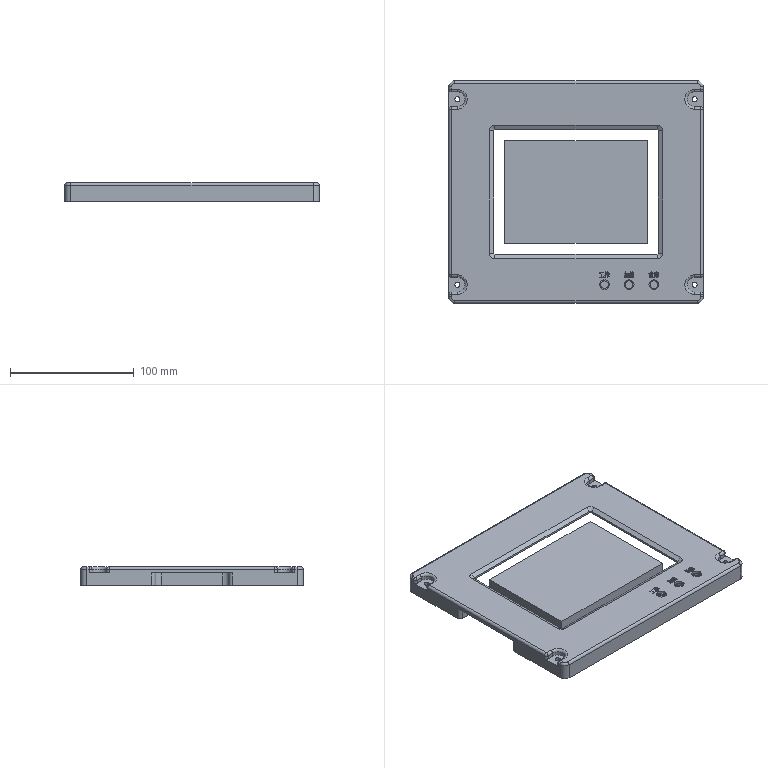NC program | Mastercam | posted with a generic post | part box 206 x 180 x 15 mm
Lines 1 to 736 of 42274:
%
:0001()
(MATERIAL - ALUMINUM MM - 2024)
(T24|100 FEM |H24)
(T9|10 FEM |H9|XY STOCK TO LEAVE - .15|Z STOCK TO LEAVE - .05)
(T10|10 FEM |H10)
(T1|4 BNOS |H1|XY STOCK TO LEAVE - .1|Z STOCK TO LEAVE - 0.)
(T14|2 BM/BNOS |H14)
(T4|4 FEM |H4|XY STOCK TO LEAVE - -.01|Z STOCK TO LEAVE - 0.)
(T8|8 FEM |H8|XY STOCK TO LEAVE - 0.|Z STOCK TO LEAVE - .1)
(T5|4 CHM |H5)
(T2|2 FEM |H2|XY STOCK TO LEAVE - .1|Z STOCK TO LEAVE - 0.)
N100 G21
N102 G0 G17 G40 G80 G90 G94 G98
N104 G0 G28 G91 Z0.
N106 G0 G28 X0. Y0.
(100 FEM |TOOL - 24|DIA. OFF. - 24|LEN. - 24|TOOL DIA. - 100.)
N108 T24 M6
N110 G0 G54 G90 X-215.5 Y64.998 C0. B0. S4000 M3
N112 G43 H24 Z51.
N114 Z3.
N116 G1 Z.55 F600.
N118 X155.5 F1000.
N120 G2 X187.999 Y32.499 J-32.499
N122 X155.5 Y0. I-32.499
N124 G1 X-155.5
N126 G3 X-187.999 Y-32.499 J-32.499
N128 X-155.5 Y-64.998 I32.499
N130 G1 X215.5
N132 G0 Z50.55
N134 X-215.5 Y64.998
N136 Z2.55
N138 G1 Z.1 F600.
N140 X155.5 F1000.
N142 G2 X187.999 Y32.499 J-32.499
N144 X155.5 Y0. I-32.499
N146 G1 X-155.5
N148 G3 X-187.999 Y-32.499 J-32.499
N150 X-155.5 Y-64.998 I32.499
N152 G1 X215.5
N154 G0 Z50.1
N156 X-215.5 Y64.998
N158 Z2.1
N160 G1 Z0. F600.
N162 X155.5 F1000.
N164 G2 X187.999 Y32.499 J-32.499
N166 X155.5 Y0. I-32.499
N168 G1 X-155.5
N170 G3 X-187.999 Y-32.499 J-32.499
N172 X-155.5 Y-64.998 I32.499
N174 G1 X215.5
N176 G0 Z50.
N178 M5
N180 G0 G28 G91 Z0.
N182 G28
N184 M01
N186 G0 G17 G40 G80 G90 G94 G98
N188 G0 G28 G91 Z0.
(10 FEM |TOOL - 9|DIA. OFF. - 9|LEN. - 9|TOOL DIA. - 10.)
N190 T9 M6
N192 G0 G54 G90 X-99. Y97.15 C0. B0. S7000 M3
N194 G43 H9 Z50.
N196 Z1.
N198 G1 Z0. F600.
N200 Y96.15 F3000.
N202 G3 X-98. Y95.15 I1.
N204 G1 X98. Z-.246
N206 G2 X108.15 Y85. Z-.266 J-10.15
N208 G1 Y-85. Z-.48
N210 G2 X98. Y-95.15 Z-.5 I-10.15
N212 G1 X-98. Z-.746
N214 G2 X-108.15 Y-85. Z-.766 J10.15
N216 G1 Y85. Z-.98
N218 G2 X-98. Y95.15 Z-1. I10.15
N220 G1 X98. Z-1.246
N222 G2 X108.15 Y85. Z-1.266 J-10.15
N224 G1 Y-85. Z-1.48
N226 G2 X98. Y-95.15 Z-1.5 I-10.15
N228 G1 X-98. Z-1.746
N230 G2 X-108.15 Y-85. Z-1.766 J10.15
N232 G1 Y85. Z-1.98
N234 G2 X-98. Y95.15 Z-2. I10.15
N236 G1 X98. Z-2.246
N238 G2 X108.15 Y85. Z-2.266 J-10.15
N240 G1 Y-85. Z-2.48
N242 G2 X98. Y-95.15 Z-2.5 I-10.15
N244 G1 X-98. Z-2.746
N246 G2 X-108.15 Y-85. Z-2.766 J10.15
N248 G1 Y85. Z-2.98
N250 G2 X-98. Y95.15 Z-3. I10.15
N252 G1 X98. Z-3.246
N254 G2 X108.15 Y85. Z-3.266 J-10.15
N256 G1 Y-85. Z-3.48
N258 G2 X98. Y-95.15 Z-3.5 I-10.15
N260 G1 X-98. Z-3.746
N262 G2 X-108.15 Y-85. Z-3.766 J10.15
N264 G1 Y85. Z-3.98
N266 G2 X-98. Y95.15 Z-4. I10.15
N268 G1 X98. Z-4.246
N270 G2 X108.15 Y85. Z-4.266 J-10.15
N272 G1 Y-85. Z-4.48
N274 G2 X98. Y-95.15 Z-4.5 I-10.15
N276 G1 X-98. Z-4.746
N278 G2 X-108.15 Y-85. Z-4.766 J10.15
N280 G1 Y85. Z-4.98
N282 G2 X-98. Y95.15 Z-5. I10.15
N284 G1 X98. Z-5.246
N286 G2 X108.15 Y85. Z-5.266 J-10.15
N288 G1 Y-85. Z-5.48
N290 G2 X98. Y-95.15 Z-5.5 I-10.15
N292 G1 X-98. Z-5.746
N294 G2 X-108.15 Y-85. Z-5.766 J10.15
N296 G1 Y85. Z-5.98
N298 G2 X-98. Y95.15 Z-6. I10.15
N300 G1 X98. Z-6.246
N302 G2 X108.15 Y85. Z-6.266 J-10.15
N304 G1 Y-85. Z-6.48
N306 G2 X98. Y-95.15 Z-6.5 I-10.15
N308 G1 X-98. Z-6.746
N310 G2 X-108.15 Y-85. Z-6.766 J10.15
N312 G1 Y85. Z-6.98
N314 G2 X-98. Y95.15 Z-7. I10.15
N316 G1 X98. Z-7.246
N318 G2 X108.15 Y85. Z-7.266 J-10.15
N320 G1 Y-85. Z-7.48
N322 G2 X98. Y-95.15 Z-7.5 I-10.15
N324 G1 X-98. Z-7.746
N326 G2 X-108.15 Y-85. Z-7.766 J10.15
N328 G1 Y85. Z-7.98
N330 G2 X-98. Y95.15 Z-8. I10.15
N332 G1 X98. Z-8.246
N334 G2 X108.15 Y85. Z-8.266 J-10.15
N336 G1 Y-85. Z-8.48
N338 G2 X98. Y-95.15 Z-8.5 I-10.15
N340 G1 X-98. Z-8.746
N342 G2 X-108.15 Y-85. Z-8.766 J10.15
N344 G1 Y85. Z-8.98
N346 G2 X-98. Y95.15 Z-9. I10.15
N348 G1 X98. Z-9.246
N350 G2 X108.15 Y85. Z-9.266 J-10.15
N352 G1 Y-85. Z-9.48
N354 G2 X98. Y-95.15 Z-9.5 I-10.15
N356 G1 X-98. Z-9.746
N358 G2 X-108.15 Y-85. Z-9.766 J10.15
N360 G1 Y85. Z-9.98
N362 G2 X-98. Y95.15 Z-10. I10.15
N364 G1 X98. Z-10.246
N366 G2 X108.15 Y85. Z-10.266 J-10.15
N368 G1 Y-85. Z-10.48
N370 G2 X98. Y-95.15 Z-10.5 I-10.15
N372 G1 X-98. Z-10.746
N374 G2 X-108.15 Y-85. Z-10.766 J10.15
N376 G1 Y85. Z-10.98
N378 G2 X-98. Y95.15 Z-11. I10.15
N380 G1 X98. Z-11.246
N382 G2 X108.15 Y85. Z-11.266 J-10.15
N384 G1 Y-85. Z-11.48
N386 G2 X98. Y-95.15 Z-11.5 I-10.15
N388 G1 X-98. Z-11.746
N390 G2 X-108.15 Y-85. Z-11.766 J10.15
N392 G1 Y85. Z-11.98
N394 G2 X-98. Y95.15 Z-12. I10.15
N396 G1 X98. Z-12.246
N398 G2 X108.15 Y85. Z-12.266 J-10.15
N400 G1 Y-85. Z-12.48
N402 G2 X98. Y-95.15 Z-12.5 I-10.15
N404 G1 X-98. Z-12.746
N406 G2 X-108.15 Y-85. Z-12.766 J10.15
N408 G1 Y85. Z-12.98
N410 G2 X-98. Y95.15 Z-13. I10.15
N412 G1 X98. Z-13.246
N414 G2 X108.15 Y85. Z-13.266 J-10.15
N416 G1 Y-85. Z-13.48
N418 G2 X98. Y-95.15 Z-13.5 I-10.15
N420 G1 X-98. Z-13.746
N422 G2 X-108.15 Y-85. Z-13.766 J10.15
N424 G1 Y85. Z-13.98
N426 G2 X-98. Y95.15 Z-14. I10.15
N428 G1 X98. Z-14.246
N430 G2 X108.15 Y85. Z-14.266 J-10.15
N432 G1 Y-85. Z-14.48
N434 G2 X98. Y-95.15 Z-14.5 I-10.15
N436 G1 X-98. Z-14.746
N438 G2 X-108.15 Y-85. Z-14.766 J10.15
N440 G1 Y61.155 Z-14.95
N442 Y85.
N444 G2 X-98. Y95.15 I10.15
N446 G1 X98.
N448 G2 X108.15 Y85. J-10.15
N450 G1 Y-85.
N452 G2 X98. Y-95.15 I-10.15
N454 G1 X-98.
N456 G2 X-108.15 Y-85. J10.15
N458 G1 Y61.155
N460 G3 X-109.15 Y62.155 I-1.
N462 G1 X-110.15
N464 G0 Z50.
N466 X-110.1 Y66.
N468 Z1.
N470 G1 Z-.485 F600.
N472 X-109.1 F3000.
N474 G3 X-108.1 Y67. J1.
N476 G2 X-101. Y74.1 I7.1
N478 G1 X-96.
N480 G3 X-95.1 Y75. J.9
N482 X-96. Y75.9 I-.9
N484 G1 X-101.
N486 G2 X-108.1 Y83. J7.1
N488 G3 X-109.1 Y84. I-1.
N490 G1 X-110.1
N492 Z-.97 F600.
N494 X-109.1 F3000.
N496 G2 X-108.1 Y83. J-1.
N498 G3 X-101. Y75.9 I7.1
N500 G1 X-96.
N502 G2 X-95.1 Y75. J-.9
N504 X-96. Y74.1 I-.9
N506 G1 X-101.
N508 G3 X-108.1 Y67. J-7.1
N510 G2 X-109.1 Y66. I-1.
N512 G1 X-110.1
N514 Z-1.455 F600.
N516 X-109.1 F3000.
N518 G3 X-108.1 Y67. J1.
N520 G2 X-101. Y74.1 I7.1
N522 G1 X-96.
N524 G3 X-95.1 Y75. J.9
N526 X-96. Y75.9 I-.9
N528 G1 X-101.
N530 G2 X-108.1 Y83. J7.1
N532 G3 X-109.1 Y84. I-1.
N534 G1 X-110.1
N536 Z-1.94 F600.
N538 X-109.1 F3000.
N540 G2 X-108.1 Y83. J-1.
N542 G3 X-101. Y75.9 I7.1
N544 G1 X-96.
N546 G2 X-95.1 Y75. J-.9
N548 X-96. Y74.1 I-.9
N550 G1 X-101.
N552 G3 X-108.1 Y67. J-7.1
N554 G2 X-109.1 Y66. I-1.
N556 G1 X-110.1
N558 Z-2.425 F600.
N560 X-109.1 F3000.
N562 G3 X-108.1 Y67. J1.
N564 G2 X-101. Y74.1 I7.1
N566 G1 X-96.
N568 G3 X-95.1 Y75. J.9
N570 X-96. Y75.9 I-.9
N572 G1 X-101.
N574 G2 X-108.1 Y83. J7.1
N576 G3 X-109.1 Y84. I-1.
N578 G1 X-110.1
N580 Z-2.91 F600.
N582 X-109.1 F3000.
N584 G2 X-108.1 Y83. J-1.
N586 G3 X-101. Y75.9 I7.1
N588 G1 X-96.
N590 G2 X-95.1 Y75. J-.9
N592 X-96. Y74.1 I-.9
N594 G1 X-101.
N596 G3 X-108.1 Y67. J-7.1
N598 G2 X-109.1 Y66. I-1.
N600 G1 X-110.1
N602 Z-3.395 F600.
N604 X-109.1 F3000.
N606 G3 X-108.1 Y67. J1.
N608 G2 X-101. Y74.1 I7.1
N610 G1 X-96.
N612 G3 X-95.1 Y75. J.9
N614 X-96. Y75.9 I-.9
N616 G1 X-101.
N618 G2 X-108.1 Y83. J7.1
N620 G3 X-109.1 Y84. I-1.
N622 G1 X-110.1
N624 Z-3.88 F600.
N626 X-109.1 F3000.
N628 G2 X-108.1 Y83. J-1.
N630 G3 X-101. Y75.9 I7.1
N632 G1 X-96.
N634 G2 X-95.1 Y75. J-.9
N636 X-96. Y74.1 I-.9
N638 G1 X-101.
N640 G3 X-108.1 Y67. J-7.1
N642 G2 X-109.1 Y66. I-1.
N644 G1 X-110.1
N646 Z-4.365 F600.
N648 X-109.1 F3000.
N650 G3 X-108.1 Y67. J1.
N652 G2 X-101. Y74.1 I7.1
N654 G1 X-96.
N656 G3 X-95.1 Y75. J.9
N658 X-96. Y75.9 I-.9
N660 G1 X-101.
N662 G2 X-108.1 Y83. J7.1
N664 G3 X-109.1 Y84. I-1.
N666 G1 X-110.1
N668 Z-4.85 F600.
N670 X-109.1 F3000.
N672 G2 X-108.1 Y83. J-1.
N674 G3 X-101. Y75.9 I7.1
N676 G1 X-96.
N678 G2 X-95.1 Y75. J-.9
N680 X-96. Y74.1 I-.9
N682 G1 X-101.
N684 G3 X-108.1 Y67. J-7.1
N686 G2 X-109.1 Y66. I-1.
N688 G1 X-110.1
N690 G0 Z50.
N692 Y-84.
N694 Z1.
N696 G1 Z-.485 F600.
N698 X-109.1 F3000.
N700 G3 X-108.1 Y-83. J1.
N702 G2 X-101. Y-75.9 I7.1
N704 G1 X-96.
N706 G3 X-95.1 Y-75. J.9
N708 X-96. Y-74.1 I-.9
N710 G1 X-101.
N712 G2 X-108.1 Y-67. J7.1
N714 G3 X-109.1 Y-66. I-1.
N716 G1 X-110.1
N718 Z-.97 F600.
N720 X-109.1 F3000.
N722 G2 X-108.1 Y-67. J-1.
N724 G3 X-101. Y-74.1 I7.1
N726 G1 X-96.
N728 G2 X-95.1 Y-75. J-.9
N730 X-96. Y-75.9 I-.9
N732 G1 X-101.
N734 G3 X-108.1 Y-83. J-7.1
N736 G2 X-109.1 Y-84. I-1.
N738 G1 X-110.1
N740 Z-1.455 F600.
N742 X-109.1 F3000.
N744 G3 X-108.1 Y-83. J1.
N746 G2 X-101. Y-75.9 I7.1
N748 G1 X-96.
N750 G3 X-95.1 Y-75. J.9
N752 X-96. Y-74.1 I-.9
N754 G1 X-101.
N756 G2 X-108.1 Y-67. J7.1
N758 G3 X-109.1 Y-66. I-1.
N760 G1 X-110.1
N762 Z-1.94 F600.
N764 X-109.1 F3000.
N766 G2 X-108.1 Y-67. J-1.
N768 G3 X-101. Y-74.1 I7.1
N770 G1 X-96.
N772 G2 X-95.1 Y-75. J-.9
N774 X-96. Y-75.9 I-.9
N776 G1 X-101.
N778 G3 X-108.1 Y-83. J-7.1
N780 G2 X-109.1 Y-84. I-1.
N782 G1 X-110.1
N784 Z-2.425 F600.
N786 X-109.1 F3000.
N788 G3 X-108.1 Y-83. J1.
N790 G2 X-101. Y-75.9 I7.1
N792 G1 X-96.
N794 G3 X-95.1 Y-75. J.9
N796 X-96. Y-74.1 I-.9
N798 G1 X-101.
N800 G2 X-108.1 Y-67. J7.1
N802 G3 X-109.1 Y-66. I-1.
N804 G1 X-110.1
N806 Z-2.91 F600.
N808 X-109.1 F3000.
N810 G2 X-108.1 Y-67. J-1.
N812 G3 X-101. Y-74.1 I7.1
N814 G1 X-96.
N816 G2 X-95.1 Y-75. J-.9
N818 X-96. Y-75.9 I-.9
N820 G1 X-101.
N822 G3 X-108.1 Y-83. J-7.1
N824 G2 X-109.1 Y-84. I-1.
N826 G1 X-110.1
N828 Z-3.395 F600.
N830 X-109.1 F3000.
N832 G3 X-108.1 Y-83. J1.
N834 G2 X-101. Y-75.9 I7.1
N836 G1 X-96.
N838 G3 X-95.1 Y-75. J.9
N840 X-96. Y-74.1 I-.9
N842 G1 X-101.
N844 G2 X-108.1 Y-67. J7.1
N846 G3 X-109.1 Y-66. I-1.
N848 G1 X-110.1
N850 Z-3.88 F600.
N852 X-109.1 F3000.
N854 G2 X-108.1 Y-67. J-1.
N856 G3 X-101. Y-74.1 I7.1
N858 G1 X-96.
N860 G2 X-95.1 Y-75. J-.9
N862 X-96. Y-75.9 I-.9
N864 G1 X-101.
N866 G3 X-108.1 Y-83. J-7.1
N868 G2 X-109.1 Y-84. I-1.
N870 G1 X-110.1
N872 Z-4.365 F600.
N874 X-109.1 F3000.
N876 G3 X-108.1 Y-83. J1.
N878 G2 X-101. Y-75.9 I7.1
N880 G1 X-96.
N882 G3 X-95.1 Y-75. J.9
N884 X-96. Y-74.1 I-.9
N886 G1 X-101.
N888 G2 X-108.1 Y-67. J7.1
N890 G3 X-109.1 Y-66. I-1.
N892 G1 X-110.1
N894 Z-4.85 F600.
N896 X-109.1 F3000.
N898 G2 X-108.1 Y-67. J-1.
N900 G3 X-101. Y-74.1 I7.1
N902 G1 X-96.
N904 G2 X-95.1 Y-75. J-.9
N906 X-96. Y-75.9 I-.9
N908 G1 X-101.
N910 G3 X-108.1 Y-83. J-7.1
N912 G2 X-109.1 Y-84. I-1.
N914 G1 X-110.1
N916 G0 Z50.
N918 X110.1 Y-66.
N920 Z1.
N922 G1 Z-.485 F600.
N924 X109.1 F3000.
N926 G3 X108.1 Y-67. J-1.
N928 G2 X101. Y-74.1 I-7.1
N930 G1 X96.
N932 G3 X95.1 Y-75. J-.9
N934 X96. Y-75.9 I.9
N936 G1 X101.
N938 G2 X108.1 Y-83. J-7.1
N940 G3 X109.1 Y-84. I1.
N942 G1 X110.1
N944 Z-.97 F600.
N946 X109.1 F3000.
N948 G2 X108.1 Y-83. J1.
N950 G3 X101. Y-75.9 I-7.1
N952 G1 X96.
N954 G2 X95.1 Y-75. J.9
N956 X96. Y-74.1 I.9
N958 G1 X101.
N960 G3 X108.1 Y-67. J7.1
N962 G2 X109.1 Y-66. I1.
N964 G1 X110.1
N966 Z-1.455 F600.
N968 X109.1 F3000.
N970 G3 X108.1 Y-67. J-1.
N972 G2 X101. Y-74.1 I-7.1
N974 G1 X96.
N976 G3 X95.1 Y-75. J-.9
N978 X96. Y-75.9 I.9
N980 G1 X101.
N982 G2 X108.1 Y-83. J-7.1
N984 G3 X109.1 Y-84. I1.
N986 G1 X110.1
N988 Z-1.94 F600.
N990 X109.1 F3000.
N992 G2 X108.1 Y-83. J1.
N994 G3 X101. Y-75.9 I-7.1
N996 G1 X96.
N998 G2 X95.1 Y-75. J.9
N1000 X96. Y-74.1 I.9
N1002 G1 X101.
N1004 G3 X108.1 Y-67. J7.1
N1006 G2 X109.1 Y-66. I1.
N1008 G1 X110.1
N1010 Z-2.425 F600.
N1012 X109.1 F3000.
N1014 G3 X108.1 Y-67. J-1.
N1016 G2 X101. Y-74.1 I-7.1
N1018 G1 X96.
N1020 G3 X95.1 Y-75. J-.9
N1022 X96. Y-75.9 I.9
N1024 G1 X101.
N1026 G2 X108.1 Y-83. J-7.1
N1028 G3 X109.1 Y-84. I1.
N1030 G1 X110.1
N1032 Z-2.91 F600.
N1034 X109.1 F3000.
N1036 G2 X108.1 Y-83. J1.
N1038 G3 X101. Y-75.9 I-7.1
N1040 G1 X96.
N1042 G2 X95.1 Y-75. J.9
N1044 X96. Y-74.1 I.9
N1046 G1 X101.
N1048 G3 X108.1 Y-67. J7.1
N1050 G2 X109.1 Y-66. I1.
N1052 G1 X110.1
N1054 Z-3.395 F600.
N1056 X109.1 F3000.
N1058 G3 X108.1 Y-67. J-1.
N1060 G2 X101. Y-74.1 I-7.1
N1062 G1 X96.
N1064 G3 X95.1 Y-75. J-.9
N1066 X96. Y-75.9 I.9
N1068 G1 X101.
N1070 G2 X108.1 Y-83. J-7.1
N1072 G3 X109.1 Y-84. I1.
N1074 G1 X110.1
N1076 Z-3.88 F600.
N1078 X109.1 F3000.
N1080 G2 X108.1 Y-83. J1.
N1082 G3 X101. Y-75.9 I-7.1
N1084 G1 X96.
N1086 G2 X95.1 Y-75. J.9
N1088 X96. Y-74.1 I.9
N1090 G1 X101.
N1092 G3 X108.1 Y-67. J7.1
N1094 G2 X109.1 Y-66. I1.
N1096 G1 X110.1
N1098 Z-4.365 F600.
N1100 X109.1 F3000.
N1102 G3 X108.1 Y-67. J-1.
N1104 G2 X101. Y-74.1 I-7.1
N1106 G1 X96.
N1108 G3 X95.1 Y-75. J-.9
N1110 X96. Y-75.9 I.9
N1112 G1 X101.
N1114 G2 X108.1 Y-83. J-7.1
N1116 G3 X109.1 Y-84. I1.
N1118 G1 X110.1
N1120 Z-4.85 F600.
N1122 X109.1 F3000.
N1124 G2 X108.1 Y-83. J1.
N1126 G3 X101. Y-75.9 I-7.1
N1128 G1 X96.
N1130 G2 X95.1 Y-75. J.9
N1132 X96. Y-74.1 I.9
N1134 G1 X101.
N1136 G3 X108.1 Y-67. J7.1
N1138 G2 X109.1 Y-66. I1.
N1140 G1 X110.1
N1142 G0 Z50.
N1144 Y84.
N1146 Z1.
N1148 G1 Z-.485 F600.
N1150 X109.1 F3000.
N1152 G3 X108.1 Y83. J-1.
N1154 G2 X101. Y75.9 I-7.1
N1156 G1 X96.
N1158 G3 X95.1 Y75. J-.9
N1160 X96. Y74.1 I.9
N1162 G1 X101.
N1164 G2 X108.1 Y67. J-7.1
N1166 G3 X109.1 Y66. I1.
N1168 G1 X110.1
N1170 Z-.97 F600.
N1172 X109.1 F3000.
N1174 G2 X108.1 Y67. J1.
N1176 G3 X101. Y74.1 I-7.1
N1178 G1 X96.
N1180 G2 X95.1 Y75. J.9
N1182 X96. Y75.9 I.9
N1184 G1 X101.
N1186 G3 X108.1 Y83. J7.1
N1188 G2 X109.1 Y84. I1.
N1190 G1 X110.1
N1192 Z-1.455 F600.
N1194 X109.1 F3000.
N1196 G3 X108.1 Y83. J-1.
N1198 G2 X101. Y75.9 I-7.1
N1200 G1 X96.
N1202 G3 X95.1 Y75. J-.9
N1204 X96. Y74.1 I.9
N1206 G1 X101.
N1208 G2 X108.1 Y67. J-7.1
N1210 G3 X109.1 Y66. I1.
N1212 G1 X110.1
N1214 Z-1.94 F600.
N1216 X109.1 F3000.
N1218 G2 X108.1 Y67. J1.
N1220 G3 X101. Y74.1 I-7.1
N1222 G1 X96.
N1224 G2 X95.1 Y75. J.9
N1226 X96. Y75.9 I.9
N1228 G1 X101.
N1230 G3 X108.1 Y83. J7.1
N1232 G2 X109.1 Y84. I1.
N1234 G1 X110.1
N1236 Z-2.425 F600.
N1238 X109.1 F3000.
N1240 G3 X108.1 Y83. J-1.
N1242 G2 X101. Y75.9 I-7.1
N1244 G1 X96.
N1246 G3 X95.1 Y75. J-.9
N1248 X96. Y74.1 I.9
N1250 G1 X101.
N1252 G2 X108.1 Y67. J-7.1
N1254 G3 X109.1 Y66. I1.
N1256 G1 X110.1
N1258 Z-2.91 F600.
N1260 X109.1 F3000.
N1262 G2 X108.1 Y67. J1.
N1264 G3 X101. Y74.1 I-7.1
N1266 G1 X96.
N1268 G2 X95.1 Y75. J.9
N1270 X96. Y75.9 I.9
N1272 G1 X101.
N1274 G3 X108.1 Y83. J7.1
N1276 G2 X109.1 Y84. I1.
N1278 G1 X110.1
N1280 Z-3.395 F600.
N1282 X109.1 F3000.
N1284 G3 X108.1 Y83. J-1.
N1286 G2 X101. Y75.9 I-7.1
N1288 G1 X96.
N1290 G3 X95.1 Y75. J-.9
N1292 X96. Y74.1 I.9
N1294 G1 X101.
N1296 G2 X108.1 Y67. J-7.1
N1298 G3 X109.1 Y66. I1.
N1300 G1 X110.1
N1302 Z-3.88 F600.
N1304 X109.1 F3000.
N1306 G2 X108.1 Y67. J1.
N1308 G3 X101. Y74.1 I-7.1
N1310 G1 X96.
N1312 G2 X95.1 Y75. J.9
N1314 X96. Y75.9 I.9
N1316 G1 X101.
N1318 G3 X108.1 Y83. J7.1
N1320 G2 X109.1 Y84. I1.
N1322 G1 X110.1
N1324 Z-4.365 F600.
N1326 X109.1 F3000.
N1328 G3 X108.1 Y83. J-1.
N1330 G2 X101. Y75.9 I-7.1
N1332 G1 X96.
N1334 G3 X95.1 Y75. J-.9
N1336 X96. Y74.1 I.9
N1338 G1 X101.
N1340 G2 X108.1 Y67. J-7.1
N1342 G3 X109.1 Y66. I1.
N1344 G1 X110.1
N1346 Z-4.85 F600.
N1348 X109.1 F3000.
N1350 G2 X108.1 Y67. J1.
N1352 G3 X101. Y74.1 I-7.1
N1354 G1 X96.
N1356 G2 X95.1 Y75. J.9
N1358 X96. Y75.9 I.9
N1360 G1 X101.
N1362 G3 X108.1 Y83. J7.1
N1364 G2 X109.1 Y84. I1.
N1366 G1 X110.1
N1368 G0 Z50.
N1370 M5
N1372 G0 G28 G91 Z0.
N1374 G28
N1376 M01
N1378 G0 G17 G40 G80 G90 G94 G98
N1380 G0 G28 G91 Z0.
(10 FEM |TOOL - 10|DIA. OFF. - 10|LEN. - 10|TOOL DIA. - 10.)
N1382 T10 M6
N1384 G0 G54 G90 X-110. Y66. C0. B0. S7000 M3
N1386 G43 H10 Z50.
N1388 Z1.
N1390 G1 Z-5. F600.
N1392 X-109. F1000.
N1394 G3 X-108. Y67. J1.
N1396 G2 X-101. Y74. I7.
N1398 G1 X-96.
N1400 G3 X-95. Y75. J1.
N1402 X-96. Y76. I-1.
N1404 G1 X-101.
N1406 G2 X-108. Y83. J7.
N1408 G3 X-109. Y84. I-1.
N1410 G1 X-110.
N1412 G0 Z50.
N1414 Y-84.
N1416 Z1.
N1418 G1 Z-5. F600.
N1420 X-109. F1000.
N1422 G3 X-108. Y-83. J1.
N1424 G2 X-101. Y-76. I7.
N1426 G1 X-96.
N1428 G3 X-95. Y-75. J1.
N1430 X-96. Y-74. I-1.
N1432 G1 X-101.
N1434 G2 X-108. Y-67. J7.
N1436 G3 X-109. Y-66. I-1.
N1438 G1 X-110.
N1440 G0 Z50.
N1442 X110.
N1444 Z1.
N1446 G1 Z-5. F600.
N1448 X109. F1000.
N1450 G3 X108. Y-67. J-1.
N1452 G2 X101. Y-74. I-7.
N1454 G1 X96.
N1456 G3 X95. Y-75. J-1.
N1458 X96. Y-76. I1.
N1460 G1 X101.
N1462 G2 X108. Y-83. J-7.
N1464 G3 X109. Y-84. I1.
N1466 G1 X110.
N1468 G0 Z50.
N1470 Y84.
N1472 Z1.
N1474 G1 Z-5. F600.
N1476 X109. F1000.
N1478 G3 X108. Y83. J-1.
N1480 G2 X101. Y76. I-7.
N1482 G1 X96.
N1484 G3 X95. Y75. J-1.
N1486 X96. Y74. I1.
N1488 G1 X101.
N1490 G2 X108. Y67. J-7.
N1492 G3 X109. Y66. I1.
N1494 G1 X110.
N1496 G0 Z50.
N1498 X-99. Y97.
N1500 Z1.
N1502 G1 Z-14.95 F600.
N1504 G41 D10 Y96. F1000.
N1506 G3 X-98. Y95. I1.
N1508 G1 X98.
N1510 G2 X108. Y85. J-10.
N1512 G1 Y-85.
N1514 G2 X98. Y-95. I-10.
N1516 G1 X-98.
N1518 G2 X-108. Y-85. J10.
N1520 G1 Y85.
N1522 G2 X-98. Y95. I10.
N1524 G3 X-97. Y96. J1.
N1526 G1 G40 Y97.
N1528 G0 Z50.
N1530 M5
N1532 G0 G28 G91 Z0.
N1534 G28
N1536 M01
N1538 G0 G17 G40 G80 G90 G94 G98
N1540 G0 G28 G91 Z0.